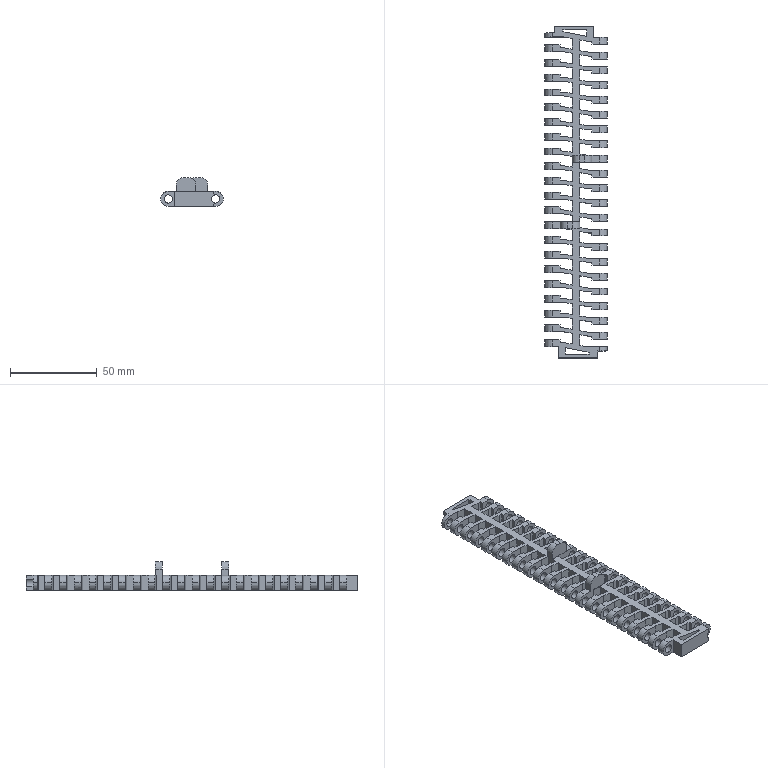Part | STEP file | 900 Mold To Width Flush Grid | 1 solid | 458 faces | box 36.002 x 191.5 x 16.69 mm | volume 24114 mm3 | plane 322 | cylinder 136 | commonest cylinder face diameters 8.74 x92 4.83 x44